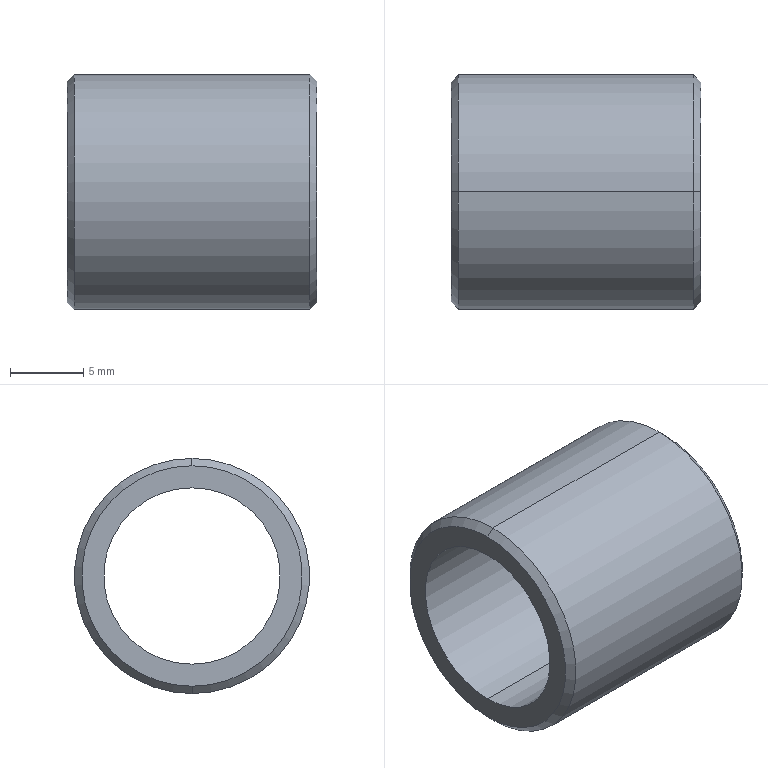Part | STEP file | CLBU12-16-3 | 1 solid | 10 faces | box 17 x 16 x 16 mm | volume 1483 mm3 | cylinder 4 | cone 4 | plane 2 | commonest cylinder face diameters 12 x2 16 x2
STEP:
#1=CARTESIAN_POINT('',(0.,0.,0.));
#2=DIRECTION('',(0.,0.,1.));
#3=DIRECTION('',(1.,0.,0.));
#4=AXIS2_PLACEMENT_3D('',#1,#2,#3);
#5=CARTESIAN_POINT('',(0.5,0.,-8.));
#6=VERTEX_POINT('',#5);
#7=CARTESIAN_POINT('',(0.5,0.,8.));
#8=VERTEX_POINT('',#7);
#9=CARTESIAN_POINT('',(0.5,0.,0.));
#10=DIRECTION('',(1.,0.,0.));
#11=DIRECTION('',(0.,0.,-1.));
#12=AXIS2_PLACEMENT_3D('',#9,#10,#11);
#13=CIRCLE('',#12,8.);
#14=CARTESIAN_POINT('',(8.5,0.,0.));
#15=DIRECTION('',(1.,0.,0.));
#16=DIRECTION('',(0.,0.,-1.));
#17=AXIS2_PLACEMENT_3D('',#14,#15,#16);
#18=CYLINDRICAL_SURFACE('',#17,8.);
#19=CARTESIAN_POINT('',(0.,-8.));
#20=DIRECTION('',(1.,0.));
#21=VECTOR('',#20,1.);
#22=LINE('',#19,#21);
#23=(GEOMETRIC_REPRESENTATION_CONTEXT(2)PARAMETRIC_REPRESENTATION_CONTEXT()REPRESENTATION_CONTEXT('',''));
#24=DEFINITIONAL_REPRESENTATION('',(#22),#23);
#25=PCURVE('',#18,#24);
#26=CARTESIAN_POINT('',(0.5,0.,0.));
#27=DIRECTION('',(1.,0.,0.));
#28=DIRECTION('',(0.,0.,-1.));
#29=AXIS2_PLACEMENT_3D('',#26,#27,#28);
#30=CONICAL_SURFACE('',#29,8.,0.7854);
#31=CARTESIAN_POINT('',(0.,0.));
#32=DIRECTION('',(1.,0.));
#33=VECTOR('',#32,1.);
#34=LINE('',#31,#33);
#35=(GEOMETRIC_REPRESENTATION_CONTEXT(2)PARAMETRIC_REPRESENTATION_CONTEXT()REPRESENTATION_CONTEXT('',''));
#36=DEFINITIONAL_REPRESENTATION('',(#34),#35);
#37=PCURVE('',#30,#36);
#38=SURFACE_CURVE('',#13,(#25,#37),.PCURVE_S1.);
#39=EDGE_CURVE('',#6,#8,#38,.T.);
#40=ORIENTED_EDGE('',*,*,#39,.T.);
#41=CARTESIAN_POINT('',(16.5,0.,8.));
#42=VERTEX_POINT('',#41);
#43=CARTESIAN_POINT('',(8.5,0.,8.));
#44=DIRECTION('',(1.,0.,0.));
#45=VECTOR('',#44,1.);
#46=LINE('',#43,#45);
#47=CARTESIAN_POINT('',(3.142,0.));
#48=DIRECTION('',(0.,1.));
#49=VECTOR('',#48,1.);
#50=LINE('',#47,#49);
#51=(GEOMETRIC_REPRESENTATION_CONTEXT(2)PARAMETRIC_REPRESENTATION_CONTEXT()REPRESENTATION_CONTEXT('',''));
#52=DEFINITIONAL_REPRESENTATION('',(#50),#51);
#53=PCURVE('',#18,#52);
#54=CARTESIAN_POINT('',(8.5,0.,0.));
#55=DIRECTION('',(1.,0.,0.));
#56=DIRECTION('',(0.,0.,-1.));
#57=AXIS2_PLACEMENT_3D('',#54,#55,#56);
#58=CYLINDRICAL_SURFACE('',#57,8.);
#59=CARTESIAN_POINT('',(3.142,0.));
#60=DIRECTION('',(0.,1.));
#61=VECTOR('',#60,1.);
#62=LINE('',#59,#61);
#63=(GEOMETRIC_REPRESENTATION_CONTEXT(2)PARAMETRIC_REPRESENTATION_CONTEXT()REPRESENTATION_CONTEXT('',''));
#64=DEFINITIONAL_REPRESENTATION('',(#62),#63);
#65=PCURVE('',#58,#64);
#66=SURFACE_CURVE('',#46,(#53,#65),.PCURVE_S1.);
#67=EDGE_CURVE('',#8,#42,#66,.T.);
#68=ORIENTED_EDGE('',*,*,#67,.T.);
#69=CARTESIAN_POINT('',(16.5,0.,-8.));
#70=VERTEX_POINT('',#69);
#71=CARTESIAN_POINT('',(16.5,0.,0.));
#72=DIRECTION('',(-1.,0.,0.));
#73=DIRECTION('',(0.,0.,-1.));
#74=AXIS2_PLACEMENT_3D('',#71,#72,#73);
#75=CIRCLE('',#74,8.);
#76=CARTESIAN_POINT('',(6.283,8.));
#77=DIRECTION('',(-1.,0.));
#78=VECTOR('',#77,1.);
#79=LINE('',#76,#78);
#80=(GEOMETRIC_REPRESENTATION_CONTEXT(2)PARAMETRIC_REPRESENTATION_CONTEXT()REPRESENTATION_CONTEXT('',''));
#81=DEFINITIONAL_REPRESENTATION('',(#79),#80);
#82=PCURVE('',#18,#81);
#83=CARTESIAN_POINT('',(16.5,0.,0.));
#84=DIRECTION('',(-1.,0.,0.));
#85=DIRECTION('',(0.,0.,1.));
#86=AXIS2_PLACEMENT_3D('',#83,#84,#85);
#87=CONICAL_SURFACE('',#86,8.,0.7854);
#88=CARTESIAN_POINT('',(-3.142,0.));
#89=DIRECTION('',(1.,0.));
#90=VECTOR('',#89,1.);
#91=LINE('',#88,#90);
#92=(GEOMETRIC_REPRESENTATION_CONTEXT(2)PARAMETRIC_REPRESENTATION_CONTEXT()REPRESENTATION_CONTEXT('',''));
#93=DEFINITIONAL_REPRESENTATION('',(#91),#92);
#94=PCURVE('',#87,#93);
#95=SURFACE_CURVE('',#75,(#82,#94),.PCURVE_S1.);
#96=EDGE_CURVE('',#42,#70,#95,.T.);
#97=ORIENTED_EDGE('',*,*,#96,.T.);
#98=CARTESIAN_POINT('',(8.5,0.,-8.));
#99=DIRECTION('',(1.,0.,0.));
#100=VECTOR('',#99,1.);
#101=LINE('',#98,#100);
#102=CARTESIAN_POINT('',(0.,0.));
#103=DIRECTION('',(0.,1.));
#104=VECTOR('',#103,1.);
#105=LINE('',#102,#104);
#106=(GEOMETRIC_REPRESENTATION_CONTEXT(2)PARAMETRIC_REPRESENTATION_CONTEXT()REPRESENTATION_CONTEXT('',''));
#107=DEFINITIONAL_REPRESENTATION('',(#105),#106);
#108=PCURVE('',#18,#107);
#109=CARTESIAN_POINT('',(6.283,0.));
#110=DIRECTION('',(0.,1.));
#111=VECTOR('',#110,1.);
#112=LINE('',#109,#111);
#113=(GEOMETRIC_REPRESENTATION_CONTEXT(2)PARAMETRIC_REPRESENTATION_CONTEXT()REPRESENTATION_CONTEXT('',''));
#114=DEFINITIONAL_REPRESENTATION('',(#112),#113);
#115=PCURVE('',#58,#114);
#116=SURFACE_CURVE('',#101,(#108,#115),.PCURVE_S1.);
#117=EDGE_CURVE('',#6,#70,#116,.T.);
#118=ORIENTED_EDGE('',*,*,#117,.F.);
#119=EDGE_LOOP('',(#40,#68,#97,#118));
#120=FACE_BOUND('',#119,.T.);
#121=ADVANCED_FACE('',(#120),#18,.T.);
#122=CARTESIAN_POINT('',(0.,0.,-7.5));
#123=VERTEX_POINT('',#122);
#124=CARTESIAN_POINT('',(0.,0.,7.5));
#125=VERTEX_POINT('',#124);
#126=CARTESIAN_POINT('',(0.,0.,0.));
#127=DIRECTION('',(1.,0.,0.));
#128=DIRECTION('',(0.,0.,-1.));
#129=AXIS2_PLACEMENT_3D('',#126,#127,#128);
#130=CIRCLE('',#129,7.5);
#131=CARTESIAN_POINT('',(0.,-0.5));
#132=DIRECTION('',(1.,0.));
#133=VECTOR('',#132,1.);
#134=LINE('',#131,#133);
#135=(GEOMETRIC_REPRESENTATION_CONTEXT(2)PARAMETRIC_REPRESENTATION_CONTEXT()REPRESENTATION_CONTEXT('',''));
#136=DEFINITIONAL_REPRESENTATION('',(#134),#135);
#137=PCURVE('',#30,#136);
#138=CARTESIAN_POINT('',(0.,6.75,0.));
#139=DIRECTION('',(-1.,0.,0.));
#140=DIRECTION('',(0.,0.,1.));
#141=AXIS2_PLACEMENT_3D('',#138,#139,#140);
#142=PLANE('',#141);
#143=CARTESIAN_POINT('',(-7.5,-6.75));
#144=CARTESIAN_POINT('',(-7.5,6.24));
#145=CARTESIAN_POINT('',(3.75,-0.2548));
#146=CARTESIAN_POINT('',(15.,-6.75));
#147=CARTESIAN_POINT('',(3.75,-13.245));
#148=CARTESIAN_POINT('',(-7.5,-19.74));
#149=CARTESIAN_POINT('',(-7.5,-6.75));
#150=(BOUNDED_CURVE()B_SPLINE_CURVE(2,(#143,#144,#145,#146,#147,#148,#149),.UNSPECIFIED.,.T.,.F.)B_SPLINE_CURVE_WITH_KNOTS((1,2,2,2,2,1),(-2.094,0.,2.094,4.189,6.283,8.378),.UNSPECIFIED.)CURVE()GEOMETRIC_REPRESENTATION_ITEM()RATIONAL_B_SPLINE_CURVE((1.,0.5,1.,0.5,1.,0.5,1.))REPRESENTATION_ITEM(''));
#151=(GEOMETRIC_REPRESENTATION_CONTEXT(2)PARAMETRIC_REPRESENTATION_CONTEXT()REPRESENTATION_CONTEXT('',''));
#152=DEFINITIONAL_REPRESENTATION('',(#150),#151);
#153=PCURVE('',#142,#152);
#154=SURFACE_CURVE('',#130,(#137,#153),.PCURVE_S1.);
#155=EDGE_CURVE('',#123,#125,#154,.T.);
#156=ORIENTED_EDGE('',*,*,#155,.T.);
#157=CARTESIAN_POINT('',(0.5,0.,8.));
#158=DIRECTION('',(0.7071,0.,0.7071));
#159=VECTOR('',#158,1.);
#160=LINE('',#157,#159);
#161=CARTESIAN_POINT('',(3.142,0.));
#162=DIRECTION('',(0.,1.));
#163=VECTOR('',#162,1.);
#164=LINE('',#161,#163);
#165=(GEOMETRIC_REPRESENTATION_CONTEXT(2)PARAMETRIC_REPRESENTATION_CONTEXT()REPRESENTATION_CONTEXT('',''));
#166=DEFINITIONAL_REPRESENTATION('',(#164),#165);
#167=PCURVE('',#30,#166);
#168=CARTESIAN_POINT('',(0.5,0.,0.));
#169=DIRECTION('',(1.,0.,0.));
#170=DIRECTION('',(0.,0.,-1.));
#171=AXIS2_PLACEMENT_3D('',#168,#169,#170);
#172=CONICAL_SURFACE('',#171,8.,0.7854);
#173=CARTESIAN_POINT('',(3.142,0.));
#174=DIRECTION('',(0.,1.));
#175=VECTOR('',#174,1.);
#176=LINE('',#173,#175);
#177=(GEOMETRIC_REPRESENTATION_CONTEXT(2)PARAMETRIC_REPRESENTATION_CONTEXT()REPRESENTATION_CONTEXT('',''));
#178=DEFINITIONAL_REPRESENTATION('',(#176),#177);
#179=PCURVE('',#172,#178);
#180=SURFACE_CURVE('',#160,(#167,#179),.PCURVE_S1.);
#181=EDGE_CURVE('',#125,#8,#180,.T.);
#182=ORIENTED_EDGE('',*,*,#181,.T.);
#183=ORIENTED_EDGE('',*,*,#39,.F.);
#184=CARTESIAN_POINT('',(0.5,0.,-8.));
#185=DIRECTION('',(0.7071,0.,-0.7071));
#186=VECTOR('',#185,1.);
#187=LINE('',#184,#186);
#188=CARTESIAN_POINT('',(0.,0.));
#189=DIRECTION('',(0.,1.));
#190=VECTOR('',#189,1.);
#191=LINE('',#188,#190);
#192=(GEOMETRIC_REPRESENTATION_CONTEXT(2)PARAMETRIC_REPRESENTATION_CONTEXT()REPRESENTATION_CONTEXT('',''));
#193=DEFINITIONAL_REPRESENTATION('',(#191),#192);
#194=PCURVE('',#30,#193);
#195=CARTESIAN_POINT('',(6.283,0.));
#196=DIRECTION('',(0.,1.));
#197=VECTOR('',#196,1.);
#198=LINE('',#195,#197);
#199=(GEOMETRIC_REPRESENTATION_CONTEXT(2)PARAMETRIC_REPRESENTATION_CONTEXT()REPRESENTATION_CONTEXT('',''));
#200=DEFINITIONAL_REPRESENTATION('',(#198),#199);
#201=PCURVE('',#172,#200);
#202=SURFACE_CURVE('',#187,(#194,#201),.PCURVE_S1.);
#203=EDGE_CURVE('',#123,#6,#202,.T.);
#204=ORIENTED_EDGE('',*,*,#203,.F.);
#205=EDGE_LOOP('',(#156,#182,#183,#204));
#206=FACE_BOUND('',#205,.T.);
#207=ADVANCED_FACE('',(#206),#30,.T.);
#208=CARTESIAN_POINT('',(17.,0.,7.5));
#209=VERTEX_POINT('',#208);
#210=CARTESIAN_POINT('',(17.,0.,-7.5));
#211=VERTEX_POINT('',#210);
#212=CARTESIAN_POINT('',(17.,0.,0.));
#213=DIRECTION('',(-1.,0.,0.));
#214=DIRECTION('',(0.,0.,1.));
#215=AXIS2_PLACEMENT_3D('',#212,#213,#214);
#216=CIRCLE('',#215,7.5);
#217=CARTESIAN_POINT('',(0.,-0.5));
#218=DIRECTION('',(1.,0.));
#219=VECTOR('',#218,1.);
#220=LINE('',#217,#219);
#221=(GEOMETRIC_REPRESENTATION_CONTEXT(2)PARAMETRIC_REPRESENTATION_CONTEXT()REPRESENTATION_CONTEXT('',''));
#222=DEFINITIONAL_REPRESENTATION('',(#220),#221);
#223=PCURVE('',#87,#222);
#224=CARTESIAN_POINT('',(17.,6.75,0.));
#225=DIRECTION('',(1.,0.,0.));
#226=DIRECTION('',(0.,0.,-1.));
#227=AXIS2_PLACEMENT_3D('',#224,#225,#226);
#228=PLANE('',#227);
#229=CARTESIAN_POINT('',(-7.5,-6.75));
#230=CARTESIAN_POINT('',(-7.5,6.24));
#231=CARTESIAN_POINT('',(3.75,-0.2548));
#232=CARTESIAN_POINT('',(15.,-6.75));
#233=CARTESIAN_POINT('',(3.75,-13.245));
#234=CARTESIAN_POINT('',(-7.5,-19.74));
#235=CARTESIAN_POINT('',(-7.5,-6.75));
#236=(BOUNDED_CURVE()B_SPLINE_CURVE(2,(#229,#230,#231,#232,#233,#234,#235),.UNSPECIFIED.,.T.,.F.)B_SPLINE_CURVE_WITH_KNOTS((1,2,2,2,2,1),(-2.094,0.,2.094,4.189,6.283,8.378),.UNSPECIFIED.)CURVE()GEOMETRIC_REPRESENTATION_ITEM()RATIONAL_B_SPLINE_CURVE((1.,0.5,1.,0.5,1.,0.5,1.))REPRESENTATION_ITEM(''));
#237=(GEOMETRIC_REPRESENTATION_CONTEXT(2)PARAMETRIC_REPRESENTATION_CONTEXT()REPRESENTATION_CONTEXT('',''));
#238=DEFINITIONAL_REPRESENTATION('',(#236),#237);
#239=PCURVE('',#228,#238);
#240=SURFACE_CURVE('',#216,(#223,#239),.PCURVE_S1.);
#241=EDGE_CURVE('',#209,#211,#240,.T.);
#242=ORIENTED_EDGE('',*,*,#241,.T.);
#243=CARTESIAN_POINT('',(16.5,0.,-8.));
#244=DIRECTION('',(-0.7071,0.,-0.7071));
#245=VECTOR('',#244,1.);
#246=LINE('',#243,#245);
#247=CARTESIAN_POINT('',(3.142,0.));
#248=DIRECTION('',(0.,1.));
#249=VECTOR('',#248,1.);
#250=LINE('',#247,#249);
#251=(GEOMETRIC_REPRESENTATION_CONTEXT(2)PARAMETRIC_REPRESENTATION_CONTEXT()REPRESENTATION_CONTEXT('',''));
#252=DEFINITIONAL_REPRESENTATION('',(#250),#251);
#253=PCURVE('',#87,#252);
#254=CARTESIAN_POINT('',(16.5,0.,0.));
#255=DIRECTION('',(-1.,0.,0.));
#256=DIRECTION('',(0.,0.,1.));
#257=AXIS2_PLACEMENT_3D('',#254,#255,#256);
#258=CONICAL_SURFACE('',#257,8.,0.7854);
#259=CARTESIAN_POINT('',(3.142,0.));
#260=DIRECTION('',(0.,1.));
#261=VECTOR('',#260,1.);
#262=LINE('',#259,#261);
#263=(GEOMETRIC_REPRESENTATION_CONTEXT(2)PARAMETRIC_REPRESENTATION_CONTEXT()REPRESENTATION_CONTEXT('',''));
#264=DEFINITIONAL_REPRESENTATION('',(#262),#263);
#265=PCURVE('',#258,#264);
#266=SURFACE_CURVE('',#246,(#253,#265),.PCURVE_S1.);
#267=EDGE_CURVE('',#211,#70,#266,.T.);
#268=ORIENTED_EDGE('',*,*,#267,.T.);
#269=ORIENTED_EDGE('',*,*,#96,.F.);
#270=CARTESIAN_POINT('',(16.5,0.,8.));
#271=DIRECTION('',(-0.7071,0.,0.7071));
#272=VECTOR('',#271,1.);
#273=LINE('',#270,#272);
#274=CARTESIAN_POINT('',(0.,0.));
#275=DIRECTION('',(0.,1.));
#276=VECTOR('',#275,1.);
#277=LINE('',#274,#276);
#278=(GEOMETRIC_REPRESENTATION_CONTEXT(2)PARAMETRIC_REPRESENTATION_CONTEXT()REPRESENTATION_CONTEXT('',''));
#279=DEFINITIONAL_REPRESENTATION('',(#277),#278);
#280=PCURVE('',#87,#279);
#281=CARTESIAN_POINT('',(6.283,0.));
#282=DIRECTION('',(0.,1.));
#283=VECTOR('',#282,1.);
#284=LINE('',#281,#283);
#285=(GEOMETRIC_REPRESENTATION_CONTEXT(2)PARAMETRIC_REPRESENTATION_CONTEXT()REPRESENTATION_CONTEXT('',''));
#286=DEFINITIONAL_REPRESENTATION('',(#284),#285);
#287=PCURVE('',#258,#286);
#288=SURFACE_CURVE('',#273,(#280,#287),.PCURVE_S1.);
#289=EDGE_CURVE('',#209,#42,#288,.T.);
#290=ORIENTED_EDGE('',*,*,#289,.F.);
#291=EDGE_LOOP('',(#242,#268,#269,#290));
#292=FACE_BOUND('',#291,.T.);
#293=ADVANCED_FACE('',(#292),#87,.T.);
#294=CARTESIAN_POINT('',(0.,0.,-6.));
#295=VERTEX_POINT('',#294);
#296=CARTESIAN_POINT('',(17.,0.,-6.));
#297=VERTEX_POINT('',#296);
#298=CARTESIAN_POINT('',(8.5,0.,-6.));
#299=DIRECTION('',(1.,0.,0.));
#300=VECTOR('',#299,1.);
#301=LINE('',#298,#300);
#302=CARTESIAN_POINT('',(8.5,0.,0.));
#303=DIRECTION('',(1.,0.,0.));
#304=DIRECTION('',(0.,0.,-1.));
#305=AXIS2_PLACEMENT_3D('',#302,#303,#304);
#306=CYLINDRICAL_SURFACE('',#305,6.);
#307=CARTESIAN_POINT('',(6.283,0.));
#308=DIRECTION('',(0.,1.));
#309=VECTOR('',#308,1.);
#310=LINE('',#307,#309);
#311=(GEOMETRIC_REPRESENTATION_CONTEXT(2)PARAMETRIC_REPRESENTATION_CONTEXT()REPRESENTATION_CONTEXT('',''));
#312=DEFINITIONAL_REPRESENTATION('',(#310),#311);
#313=PCURVE('',#306,#312);
#314=CARTESIAN_POINT('',(8.5,0.,0.));
#315=DIRECTION('',(1.,0.,0.));
#316=DIRECTION('',(0.,0.,-1.));
#317=AXIS2_PLACEMENT_3D('',#314,#315,#316);
#318=CYLINDRICAL_SURFACE('',#317,6.);
#319=CARTESIAN_POINT('',(0.,0.));
#320=DIRECTION('',(0.,1.));
#321=VECTOR('',#320,1.);
#322=LINE('',#319,#321);
#323=(GEOMETRIC_REPRESENTATION_CONTEXT(2)PARAMETRIC_REPRESENTATION_CONTEXT()REPRESENTATION_CONTEXT('',''));
#324=DEFINITIONAL_REPRESENTATION('',(#322),#323);
#325=PCURVE('',#318,#324);
#326=SURFACE_CURVE('',#301,(#313,#325),.PCURVE_S1.);
#327=EDGE_CURVE('',#295,#297,#326,.T.);
#328=ORIENTED_EDGE('',*,*,#327,.T.);
#329=CARTESIAN_POINT('',(17.,0.,6.));
#330=VERTEX_POINT('',#329);
#331=CARTESIAN_POINT('',(17.,0.,0.));
#332=DIRECTION('',(-1.,0.,0.));
#333=DIRECTION('',(0.,0.,-1.));
#334=AXIS2_PLACEMENT_3D('',#331,#332,#333);
#335=CIRCLE('',#334,6.);
#336=CARTESIAN_POINT('',(6.283,8.5));
#337=DIRECTION('',(-1.,0.));
#338=VECTOR('',#337,1.);
#339=LINE('',#336,#338);
#340=(GEOMETRIC_REPRESENTATION_CONTEXT(2)PARAMETRIC_REPRESENTATION_CONTEXT()REPRESENTATION_CONTEXT('',''));
#341=DEFINITIONAL_REPRESENTATION('',(#339),#340);
#342=PCURVE('',#306,#341);
#343=CARTESIAN_POINT('',(6.,-6.75));
#344=CARTESIAN_POINT('',(6.,-17.142));
#345=CARTESIAN_POINT('',(-3.,-11.946));
#346=CARTESIAN_POINT('',(-12.,-6.75));
#347=CARTESIAN_POINT('',(-3.,-1.554));
#348=CARTESIAN_POINT('',(6.,3.642));
#349=CARTESIAN_POINT('',(6.,-6.75));
#350=(BOUNDED_CURVE()B_SPLINE_CURVE(2,(#343,#344,#345,#346,#347,#348,#349),.UNSPECIFIED.,.T.,.F.)B_SPLINE_CURVE_WITH_KNOTS((1,2,2,2,2,1),(-2.094,0.,2.094,4.189,6.283,8.378),.UNSPECIFIED.)CURVE()GEOMETRIC_REPRESENTATION_ITEM()RATIONAL_B_SPLINE_CURVE((1.,0.5,1.,0.5,1.,0.5,1.))REPRESENTATION_ITEM(''));
#351=(GEOMETRIC_REPRESENTATION_CONTEXT(2)PARAMETRIC_REPRESENTATION_CONTEXT()REPRESENTATION_CONTEXT('',''));
#352=DEFINITIONAL_REPRESENTATION('',(#350),#351);
#353=PCURVE('',#228,#352);
#354=SURFACE_CURVE('',#335,(#342,#353),.PCURVE_S1.);
#355=EDGE_CURVE('',#297,#330,#354,.T.);
#356=ORIENTED_EDGE('',*,*,#355,.T.);
#357=CARTESIAN_POINT('',(0.,0.,6.));
#358=VERTEX_POINT('',#357);
#359=CARTESIAN_POINT('',(8.5,0.,6.));
#360=DIRECTION('',(1.,0.,0.));
#361=VECTOR('',#360,1.);
#362=LINE('',#359,#361);
#363=CARTESIAN_POINT('',(3.142,0.));
#364=DIRECTION('',(0.,1.));
#365=VECTOR('',#364,1.);
#366=LINE('',#363,#365);
#367=(GEOMETRIC_REPRESENTATION_CONTEXT(2)PARAMETRIC_REPRESENTATION_CONTEXT()REPRESENTATION_CONTEXT('',''));
#368=DEFINITIONAL_REPRESENTATION('',(#366),#367);
#369=PCURVE('',#306,#368);
#370=CARTESIAN_POINT('',(3.142,0.));
#371=DIRECTION('',(0.,1.));
#372=VECTOR('',#371,1.);
#373=LINE('',#370,#372);
#374=(GEOMETRIC_REPRESENTATION_CONTEXT(2)PARAMETRIC_REPRESENTATION_CONTEXT()REPRESENTATION_CONTEXT('',''));
#375=DEFINITIONAL_REPRESENTATION('',(#373),#374);
#376=PCURVE('',#318,#375);
#377=SURFACE_CURVE('',#362,(#369,#376),.PCURVE_S1.);
#378=EDGE_CURVE('',#358,#330,#377,.T.);
#379=ORIENTED_EDGE('',*,*,#378,.F.);
#380=CARTESIAN_POINT('',(0.,0.,0.));
#381=DIRECTION('',(1.,0.,0.));
#382=DIRECTION('',(0.,0.,-1.));
#383=AXIS2_PLACEMENT_3D('',#380,#381,#382);
#384=CIRCLE('',#383,6.);
#385=CARTESIAN_POINT('',(0.,-8.5));
#386=DIRECTION('',(1.,0.));
#387=VECTOR('',#386,1.);
#388=LINE('',#385,#387);
#389=(GEOMETRIC_REPRESENTATION_CONTEXT(2)PARAMETRIC_REPRESENTATION_CONTEXT()REPRESENTATION_CONTEXT('',''));
#390=DEFINITIONAL_REPRESENTATION('',(#388),#389);
#391=PCURVE('',#306,#390);
#392=CARTESIAN_POINT('',(-6.,-6.75));
#393=CARTESIAN_POINT('',(-6.,3.642));
#394=CARTESIAN_POINT('',(3.,-1.554));
#395=CARTESIAN_POINT('',(12.,-6.75));
#396=CARTESIAN_POINT('',(3.,-11.946));
#397=CARTESIAN_POINT('',(-6.,-17.142));
#398=CARTESIAN_POINT('',(-6.,-6.75));
#399=(BOUNDED_CURVE()B_SPLINE_CURVE(2,(#392,#393,#394,#395,#396,#397,#398),.UNSPECIFIED.,.T.,.F.)B_SPLINE_CURVE_WITH_KNOTS((1,2,2,2,2,1),(-2.094,0.,2.094,4.189,6.283,8.378),.UNSPECIFIED.)CURVE()GEOMETRIC_REPRESENTATION_ITEM()RATIONAL_B_SPLINE_CURVE((1.,0.5,1.,0.5,1.,0.5,1.))REPRESENTATION_ITEM(''));
#400=(GEOMETRIC_REPRESENTATION_CONTEXT(2)PARAMETRIC_REPRESENTATION_CONTEXT()REPRESENTATION_CONTEXT('',''));
#401=DEFINITIONAL_REPRESENTATION('',(#399),#400);
#402=PCURVE('',#142,#401);
#403=SURFACE_CURVE('',#384,(#391,#402),.PCURVE_S1.);
#404=EDGE_CURVE('',#358,#295,#403,.T.);
#405=ORIENTED_EDGE('',*,*,#404,.T.);
#406=EDGE_LOOP('',(#328,#356,#379,#405));
#407=FACE_BOUND('',#406,.F.);
#408=ADVANCED_FACE('',(#407),#306,.F.);
#409=ORIENTED_EDGE('',*,*,#67,.F.);
#410=CARTESIAN_POINT('',(0.5,0.,0.));
#411=DIRECTION('',(1.,0.,0.));
#412=DIRECTION('',(0.,0.,-1.));
#413=AXIS2_PLACEMENT_3D('',#410,#411,#412);
#414=CIRCLE('',#413,8.);
#415=CARTESIAN_POINT('',(0.,-8.));
#416=DIRECTION('',(1.,0.));
#417=VECTOR('',#416,1.);
#418=LINE('',#415,#417);
#419=(GEOMETRIC_REPRESENTATION_CONTEXT(2)PARAMETRIC_REPRESENTATION_CONTEXT()REPRESENTATION_CONTEXT('',''));
#420=DEFINITIONAL_REPRESENTATION('',(#418),#419);
#421=PCURVE('',#58,#420);
#422=CARTESIAN_POINT('',(0.,0.));
#423=DIRECTION('',(1.,0.));
#424=VECTOR('',#423,1.);
#425=LINE('',#422,#424);
#426=(GEOMETRIC_REPRESENTATION_CONTEXT(2)PARAMETRIC_REPRESENTATION_CONTEXT()REPRESENTATION_CONTEXT('',''));
#427=DEFINITIONAL_REPRESENTATION('',(#425),#426);
#428=PCURVE('',#172,#427);
#429=SURFACE_CURVE('',#414,(#421,#428),.PCURVE_S1.);
#430=EDGE_CURVE('',#8,#6,#429,.T.);
#431=ORIENTED_EDGE('',*,*,#430,.T.);
#432=ORIENTED_EDGE('',*,*,#117,.T.);
#433=CARTESIAN_POINT('',(16.5,0.,0.));
#434=DIRECTION('',(-1.,0.,0.));
#435=DIRECTION('',(0.,0.,-1.));
#436=AXIS2_PLACEMENT_3D('',#433,#434,#435);
#437=CIRCLE('',#436,8.);
#438=CARTESIAN_POINT('',(6.283,8.));
#439=DIRECTION('',(-1.,0.));
#440=VECTOR('',#439,1.);
#441=LINE('',#438,#440);
#442=(GEOMETRIC_REPRESENTATION_CONTEXT(2)PARAMETRIC_REPRESENTATION_CONTEXT()REPRESENTATION_CONTEXT('',''));
#443=DEFINITIONAL_REPRESENTATION('',(#441),#442);
#444=PCURVE('',#58,#443);
#445=CARTESIAN_POINT('',(3.142,0.));
#446=DIRECTION('',(1.,0.));
#447=VECTOR('',#446,1.);
#448=LINE('',#445,#447);
#449=(GEOMETRIC_REPRESENTATION_CONTEXT(2)PARAMETRIC_REPRESENTATION_CONTEXT()REPRESENTATION_CONTEXT('',''));
#450=DEFINITIONAL_REPRESENTATION('',(#448),#449);
#451=PCURVE('',#258,#450);
#452=SURFACE_CURVE('',#437,(#444,#451),.PCURVE_S1.);
#453=EDGE_CURVE('',#70,#42,#452,.T.);
#454=ORIENTED_EDGE('',*,*,#453,.T.);
#455=EDGE_LOOP('',(#409,#431,#432,#454));
#456=FACE_BOUND('',#455,.T.);
#457=ADVANCED_FACE('',(#456),#58,.T.);
#458=ORIENTED_EDGE('',*,*,#181,.F.);
#459=CARTESIAN_POINT('',(0.,0.,0.));
#460=DIRECTION('',(1.,0.,0.));
#461=DIRECTION('',(0.,0.,-1.));
#462=AXIS2_PLACEMENT_3D('',#459,#460,#461);
#463=CIRCLE('',#462,7.5);
#464=CARTESIAN_POINT('',(0.,-0.5));
#465=DIRECTION('',(1.,0.));
#466=VECTOR('',#465,1.);
#467=LINE('',#464,#466);
#468=(GEOMETRIC_REPRESENTATION_CONTEXT(2)PARAMETRIC_REPRESENTATION_CONTEXT()REPRESENTATION_CONTEXT('',''));
#469=DEFINITIONAL_REPRESENTATION('',(#467),#468);
#470=PCURVE('',#172,#469);
#471=CARTESIAN_POINT('',(-7.5,-6.75));
#472=CARTESIAN_POINT('',(-7.5,6.24));
#473=CARTESIAN_POINT('',(3.75,-0.2548));
#474=CARTESIAN_POINT('',(15.,-6.75));
#475=CARTESIAN_POINT('',(3.75,-13.245));
#476=CARTESIAN_POINT('',(-7.5,-19.74));
#477=CARTESIAN_POINT('',(-7.5,-6.75));
#478=(BOUNDED_CURVE()B_SPLINE_CURVE(2,(#471,#472,#473,#474,#475,#476,#477),.UNSPECIFIED.,.T.,.F.)B_SPLINE_CURVE_WITH_KNOTS((1,2,2,2,2,1),(-2.094,0.,2.094,4.189,6.283,8.378),.UNSPECIFIED.)CURVE()GEOMETRIC_REPRESENTATION_ITEM()RATIONAL_B_SPLINE_CURVE((1.,0.5,1.,0.5,1.,0.5,1.))REPRESENTATION_ITEM(''));
#479=(GEOMETRIC_REPRESENTATION_CONTEXT(2)PARAMETRIC_REPRESENTATION_CONTEXT()REPRESENTATION_CONTEXT('',''));
#480=DEFINITIONAL_REPRESENTATION('',(#478),#479);
#481=PCURVE('',#142,#480);
#482=SURFACE_CURVE('',#463,(#470,#481),.PCURVE_S1.);
#483=EDGE_CURVE('',#125,#123,#482,.T.);
#484=ORIENTED_EDGE('',*,*,#483,.T.);
#485=ORIENTED_EDGE('',*,*,#203,.T.);
#486=ORIENTED_EDGE('',*,*,#430,.F.);
#487=EDGE_LOOP('',(#458,#484,#485,#486));
#488=FACE_BOUND('',#487,.T.);
#489=ADVANCED_FACE('',(#488),#172,.T.);
#490=ORIENTED_EDGE('',*,*,#267,.F.);
#491=CARTESIAN_POINT('',(17.,0.,0.));
#492=DIRECTION('',(-1.,0.,0.));
#493=DIRECTION('',(0.,0.,1.));
#494=AXIS2_PLACEMENT_3D('',#491,#492,#493);
#495=CIRCLE('',#494,7.5);
#496=CARTESIAN_POINT('',(0.,-0.5));
#497=DIRECTION('',(1.,0.));
#498=VECTOR('',#497,1.);
#499=LINE('',#496,#498);
#500=(GEOMETRIC_REPRESENTATION_CONTEXT(2)PARAMETRIC_REPRESENTATION_CONTEXT()REPRESENTATION_CONTEXT('',''));
#501=DEFINITIONAL_REPRESENTATION('',(#499),#500);
#502=PCURVE('',#258,#501);
#503=CARTESIAN_POINT('',(-7.5,-6.75));
#504=CARTESIAN_POINT('',(-7.5,6.24));
#505=CARTESIAN_POINT('',(3.75,-0.2548));
#506=CARTESIAN_POINT('',(15.,-6.75));
#507=CARTESIAN_POINT('',(3.75,-13.245));
#508=CARTESIAN_POINT('',(-7.5,-19.74));
#509=CARTESIAN_POINT('',(-7.5,-6.75));
#510=(BOUNDED_CURVE()B_SPLINE_CURVE(2,(#503,#504,#505,#506,#507,#508,#509),.UNSPECIFIED.,.T.,.F.)B_SPLINE_CURVE_WITH_KNOTS((1,2,2,2,2,1),(-2.094,0.,2.094,4.189,6.283,8.378),.UNSPECIFIED.)CURVE()GEOMETRIC_REPRESENTATION_ITEM()RATIONAL_B_SPLINE_CURVE((1.,0.5,1.,0.5,1.,0.5,1.))REPRESENTATION_ITEM(''));
#511=(GEOMETRIC_REPRESENTATION_CONTEXT(2)PARAMETRIC_REPRESENTATION_CONTEXT()REPRESENTATION_CONTEXT('',''));
#512=DEFINITIONAL_REPRESENTATION('',(#510),#511);
#513=PCURVE('',#228,#512);
#514=SURFACE_CURVE('',#495,(#502,#513),.PCURVE_S1.);
#515=EDGE_CURVE('',#211,#209,#514,.T.);
#516=ORIENTED_EDGE('',*,*,#515,.T.);
#517=ORIENTED_EDGE('',*,*,#289,.T.);
#518=ORIENTED_EDGE('',*,*,#453,.F.);
#519=EDGE_LOOP('',(#490,#516,#517,#518));
#520=FACE_BOUND('',#519,.T.);
#521=ADVANCED_FACE('',(#520),#258,.T.);
#522=ORIENTED_EDGE('',*,*,#155,.F.);
#523=ORIENTED_EDGE('',*,*,#483,.F.);
#524=EDGE_LOOP('',(#522,#523));
#525=FACE_BOUND('',#524,.T.);
#526=CARTESIAN_POINT('',(0.,0.,0.));
#527=DIRECTION('',(1.,0.,0.));
#528=DIRECTION('',(0.,0.,-1.));
#529=AXIS2_PLACEMENT_3D('',#526,#527,#528);
#530=CIRCLE('',#529,6.);
#531=CARTESIAN_POINT('',(-6.,-6.75));
#532=CARTESIAN_POINT('',(-6.,3.642));
#533=CARTESIAN_POINT('',(3.,-1.554));
#534=CARTESIAN_POINT('',(12.,-6.75));
#535=CARTESIAN_POINT('',(3.,-11.946));
#536=CARTESIAN_POINT('',(-6.,-17.142));
#537=CARTESIAN_POINT('',(-6.,-6.75));
#538=(BOUNDED_CURVE()B_SPLINE_CURVE(2,(#531,#532,#533,#534,#535,#536,#537),.UNSPECIFIED.,.T.,.F.)B_SPLINE_CURVE_WITH_KNOTS((1,2,2,2,2,1),(-2.094,0.,2.094,4.189,6.283,8.378),.UNSPECIFIED.)CURVE()GEOMETRIC_REPRESENTATION_ITEM()RATIONAL_B_SPLINE_CURVE((1.,0.5,1.,0.5,1.,0.5,1.))REPRESENTATION_ITEM(''));
#539=(GEOMETRIC_REPRESENTATION_CONTEXT(2)PARAMETRIC_REPRESENTATION_CONTEXT()REPRESENTATION_CONTEXT('',''));
#540=DEFINITIONAL_REPRESENTATION('',(#538),#539);
#541=PCURVE('',#142,#540);
#542=CARTESIAN_POINT('',(0.,-8.5));
#543=DIRECTION('',(1.,0.));
#544=VECTOR('',#543,1.);
#545=LINE('',#542,#544);
#546=(GEOMETRIC_REPRESENTATION_CONTEXT(2)PARAMETRIC_REPRESENTATION_CONTEXT()REPRESENTATION_CONTEXT('',''));
#547=DEFINITIONAL_REPRESENTATION('',(#545),#546);
#548=PCURVE('',#318,#547);
#549=SURFACE_CURVE('',#530,(#541,#548),.PCURVE_S1.);
#550=EDGE_CURVE('',#295,#358,#549,.T.);
#551=ORIENTED_EDGE('',*,*,#550,.T.);
#552=ORIENTED_EDGE('',*,*,#404,.T.);
#553=EDGE_LOOP('',(#551,#552));
#554=FACE_BOUND('',#553,.T.);
#555=ADVANCED_FACE('',(#525,#554),#142,.T.);
#556=ORIENTED_EDGE('',*,*,#355,.T.);
#557=CARTESIAN_POINT('',(17.,0.,0.));
#558=DIRECTION('',(-1.,0.,0.));
#559=DIRECTION('',(0.,0.,-1.));
#560=AXIS2_PLACEMENT_3D('',#557,#558,#559);
#561=CIRCLE('',#560,6.);
#562=CARTESIAN_POINT('',(6.,-6.75));
#563=CARTESIAN_POINT('',(6.,-17.142));
#564=CARTESIAN_POINT('',(-3.,-11.946));
#565=CARTESIAN_POINT('',(-12.,-6.75));
#566=CARTESIAN_POINT('',(-3.,-1.554));
#567=CARTESIAN_POINT('',(6.,3.642));
#568=CARTESIAN_POINT('',(6.,-6.75));
#569=(BOUNDED_CURVE()B_SPLINE_CURVE(2,(#562,#563,#564,#565,#566,#567,#568),.UNSPECIFIED.,.T.,.F.)B_SPLINE_CURVE_WITH_KNOTS((1,2,2,2,2,1),(-2.094,0.,2.094,4.189,6.283,8.378),.UNSPECIFIED.)CURVE()GEOMETRIC_REPRESENTATION_ITEM()RATIONAL_B_SPLINE_CURVE((1.,0.5,1.,0.5,1.,0.5,1.))REPRESENTATION_ITEM(''));
#570=(GEOMETRIC_REPRESENTATION_CONTEXT(2)PARAMETRIC_REPRESENTATION_CONTEXT()REPRESENTATION_CONTEXT('',''));
#571=DEFINITIONAL_REPRESENTATION('',(#569),#570);
#572=PCURVE('',#228,#571);
#573=CARTESIAN_POINT('',(6.283,8.5));
#574=DIRECTION('',(-1.,0.));
#575=VECTOR('',#574,1.);
#576=LINE('',#573,#575);
#577=(GEOMETRIC_REPRESENTATION_CONTEXT(2)PARAMETRIC_REPRESENTATION_CONTEXT()REPRESENTATION_CONTEXT('',''));
#578=DEFINITIONAL_REPRESENTATION('',(#576),#577);
#579=PCURVE('',#318,#578);
#580=SURFACE_CURVE('',#561,(#572,#579),.PCURVE_S1.);
#581=EDGE_CURVE('',#330,#297,#580,.T.);
#582=ORIENTED_EDGE('',*,*,#581,.T.);
#583=EDGE_LOOP('',(#556,#582));
#584=FACE_BOUND('',#583,.T.);
#585=ORIENTED_EDGE('',*,*,#241,.F.);
#586=ORIENTED_EDGE('',*,*,#515,.F.);
#587=EDGE_LOOP('',(#585,#586));
#588=FACE_BOUND('',#587,.T.);
#589=ADVANCED_FACE('',(#584,#588),#228,.T.);
#590=ORIENTED_EDGE('',*,*,#581,.T.);
#591=ORIENTED_EDGE('',*,*,#327,.F.);
#592=ORIENTED_EDGE('',*,*,#550,.T.);
#593=ORIENTED_EDGE('',*,*,#378,.T.);
#594=EDGE_LOOP('',(#590,#591,#592,#593));
#595=FACE_BOUND('',#594,.F.);
#596=ADVANCED_FACE('',(#595),#318,.F.);
#597=CLOSED_SHELL('',(#121,#207,#293,#408,#457,#489,#521,#555,#589,#596));
#598=MANIFOLD_SOLID_BREP('',#597);
#599=(LENGTH_UNIT()NAMED_UNIT(*)SI_UNIT(.MILLI.,.METRE.));
#600=UNCERTAINTY_MEASURE_WITH_UNIT(LENGTH_MEASURE(0.0000001),#599,'','');
#601=(NAMED_UNIT(*)PLANE_ANGLE_UNIT()SI_UNIT($,.RADIAN.));
#602=(NAMED_UNIT(*)SI_UNIT($,.STERADIAN.)SOLID_ANGLE_UNIT());
#603=(GEOMETRIC_REPRESENTATION_CONTEXT(3)GLOBAL_UNCERTAINTY_ASSIGNED_CONTEXT((#600))GLOBAL_UNIT_ASSIGNED_CONTEXT((#599,#601,#602))REPRESENTATION_CONTEXT('',''));
#604=ADVANCED_BREP_SHAPE_REPRESENTATION('',(#4,#598),#603);